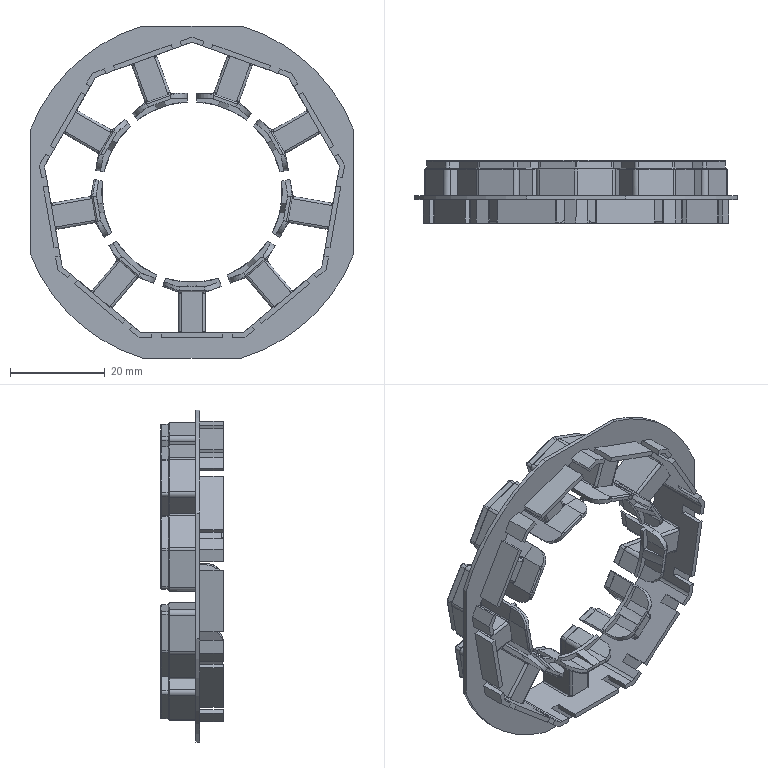Part | STEP file | SHANGHUTAO_14_1 | 1 solid | 869 faces | box 68 x 13.2 x 70 mm | volume 4829 mm3 | plane 501 | cylinder 213 | cone 99 | torus 56 | commonest cylinder face diameters 0.6 x47 1.2 x45 2 x45 1 x36 7 x18 2.4 x9